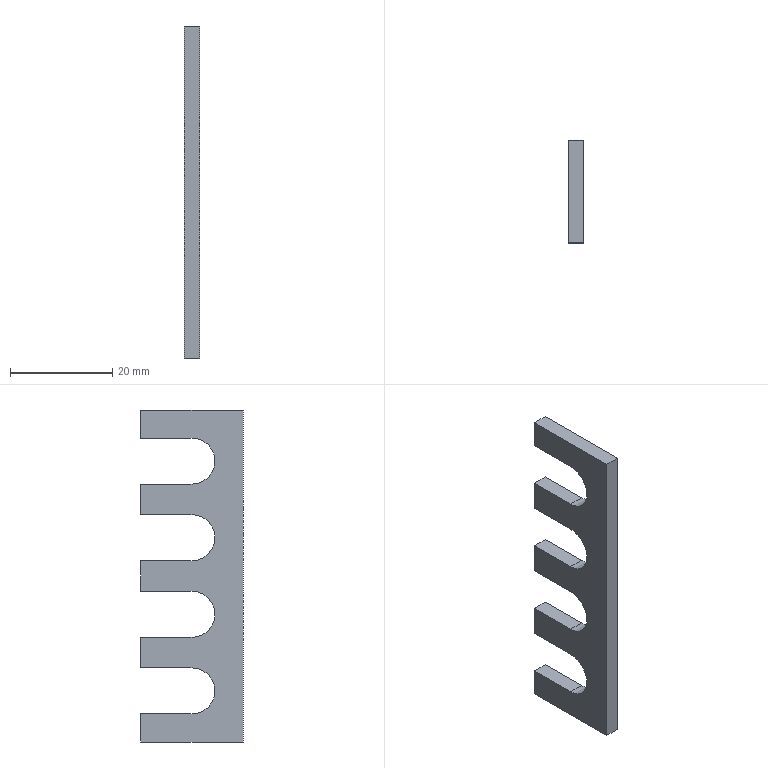Part | STEP file | Positioning_id1586_x_t | 1 solid | 22 faces | box 3 x 20 x 65 mm | volume 2438 mm3 | plane 18 | cylinder 4 | commonest cylinder face diameters 9 x4